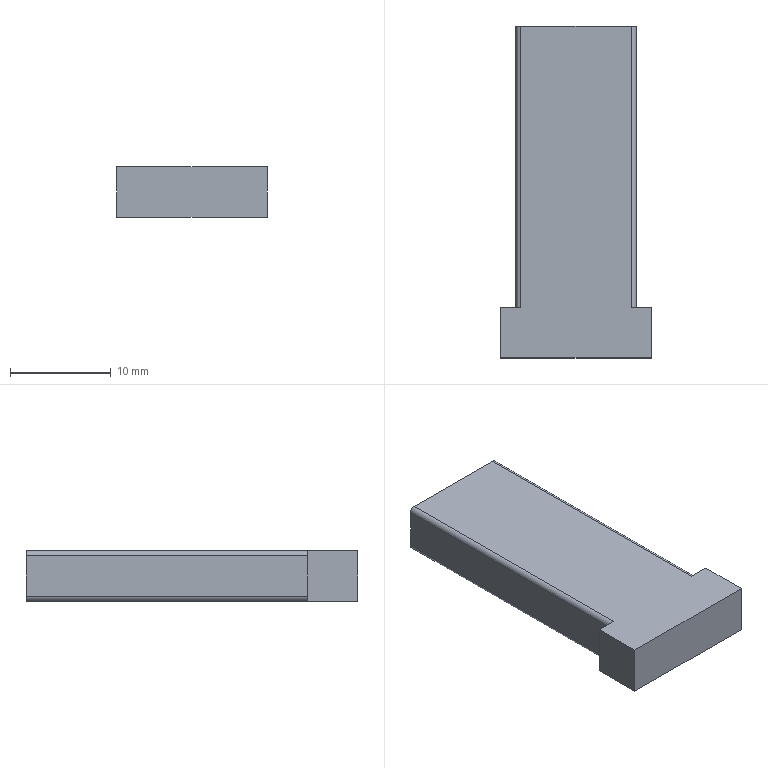Part | SolidWorks | features Extrusion 1, Fillet 1, ICE 1 | 1 solid | 14 faces | box 15 x 33 x 5 mm | volume 2049 mm3 | plane 10 | cylinder 4 | commonest cylinder face diameters 1 x4
STEP:
#1=CARTESIAN_POINT('',(-6.,-49.77,-2.));
#2=VERTEX_POINT('',#1);
#3=CARTESIAN_POINT('',(-6.,-49.77,2.));
#4=VERTEX_POINT('',#3);
#5=CARTESIAN_POINT('',(-6.,-49.77,2.5));
#6=DIRECTION('',(0.,0.,1.));
#7=VECTOR('',#6,1000.);
#8=LINE('',#5,#7);
#9=EDGE_CURVE('',#2,#4,#8,.T.);
#10=ORIENTED_EDGE('',*,*,#9,.F.);
#11=CARTESIAN_POINT('',(-5.5,-49.77,-2.5));
#12=VERTEX_POINT('',#11);
#13=CARTESIAN_POINT('',(-5.5,-49.77,-2.));
#14=DIRECTION('',(0.,-1.,0.));
#15=DIRECTION('',(0.,0.,-1.));
#16=AXIS2_PLACEMENT_3D('',#13,#14,#15);
#17=CIRCLE('',#16,0.5);
#18=EDGE_CURVE('',#2,#12,#17,.T.);
#19=ORIENTED_EDGE('',*,*,#18,.T.);
#20=CARTESIAN_POINT('',(-7.5,-49.77,-2.5));
#21=VERTEX_POINT('',#20);
#22=CARTESIAN_POINT('',(7.5,-49.77,-2.5));
#23=DIRECTION('',(-1.,0.,0.));
#24=VECTOR('',#23,1000.);
#25=LINE('',#22,#24);
#26=EDGE_CURVE('',#12,#21,#25,.T.);
#27=ORIENTED_EDGE('',*,*,#26,.T.);
#28=CARTESIAN_POINT('',(-7.5,-49.77,2.5));
#29=VERTEX_POINT('',#28);
#30=CARTESIAN_POINT('',(-7.5,-49.77,2.5));
#31=DIRECTION('',(0.,0.,-1.));
#32=VECTOR('',#31,1000.);
#33=LINE('',#30,#32);
#34=EDGE_CURVE('',#29,#21,#33,.T.);
#35=ORIENTED_EDGE('',*,*,#34,.F.);
#36=CARTESIAN_POINT('',(-5.5,-49.77,2.5));
#37=VERTEX_POINT('',#36);
#38=CARTESIAN_POINT('',(7.5,-49.77,2.5));
#39=DIRECTION('',(-1.,0.,0.));
#40=VECTOR('',#39,1000.);
#41=LINE('',#38,#40);
#42=EDGE_CURVE('',#37,#29,#41,.T.);
#43=ORIENTED_EDGE('',*,*,#42,.F.);
#44=CARTESIAN_POINT('',(-5.5,-49.77,2.));
#45=DIRECTION('',(0.,-1.,0.));
#46=DIRECTION('',(0.,0.,-1.));
#47=AXIS2_PLACEMENT_3D('',#44,#45,#46);
#48=CIRCLE('',#47,0.5);
#49=EDGE_CURVE('',#37,#4,#48,.T.);
#50=ORIENTED_EDGE('',*,*,#49,.T.);
#51=EDGE_LOOP('',(#10,#19,#27,#35,#43,#50));
#52=FACE_OUTER_BOUND('',#51,.T.);
#53=CARTESIAN_POINT('',(7.5,-49.77,2.5));
#54=DIRECTION('',(0.,-1.,0.));
#55=DIRECTION('',(0.,0.,-1.));
#56=AXIS2_PLACEMENT_3D('',#53,#54,#55);
#57=PLANE('',#56);
#58=ADVANCED_FACE('',(#52),#57,.F.);
#59=CARTESIAN_POINT('',(6.,-49.77,2.));
#60=VERTEX_POINT('',#59);
#61=CARTESIAN_POINT('',(6.,-49.77,-2.));
#62=VERTEX_POINT('',#61);
#63=CARTESIAN_POINT('',(6.,-49.77,2.5));
#64=DIRECTION('',(0.,0.,-1.));
#65=VECTOR('',#64,1000.);
#66=LINE('',#63,#65);
#67=EDGE_CURVE('',#60,#62,#66,.T.);
#68=ORIENTED_EDGE('',*,*,#67,.F.);
#69=CARTESIAN_POINT('',(5.5,-49.77,2.5));
#70=VERTEX_POINT('',#69);
#71=CARTESIAN_POINT('',(5.5,-49.77,2.));
#72=DIRECTION('',(0.,-1.,0.));
#73=DIRECTION('',(0.,0.,-1.));
#74=AXIS2_PLACEMENT_3D('',#71,#72,#73);
#75=CIRCLE('',#74,0.5);
#76=EDGE_CURVE('',#60,#70,#75,.T.);
#77=ORIENTED_EDGE('',*,*,#76,.T.);
#78=CARTESIAN_POINT('',(7.5,-49.77,2.5));
#79=VERTEX_POINT('',#78);
#80=CARTESIAN_POINT('',(7.5,-49.77,2.5));
#81=DIRECTION('',(-1.,0.,0.));
#82=VECTOR('',#81,1000.);
#83=LINE('',#80,#82);
#84=EDGE_CURVE('',#79,#70,#83,.T.);
#85=ORIENTED_EDGE('',*,*,#84,.F.);
#86=CARTESIAN_POINT('',(7.5,-49.77,-2.5));
#87=VERTEX_POINT('',#86);
#88=CARTESIAN_POINT('',(7.5,-49.77,2.5));
#89=DIRECTION('',(0.,0.,-1.));
#90=VECTOR('',#89,1000.);
#91=LINE('',#88,#90);
#92=EDGE_CURVE('',#79,#87,#91,.T.);
#93=ORIENTED_EDGE('',*,*,#92,.T.);
#94=CARTESIAN_POINT('',(5.5,-49.77,-2.5));
#95=VERTEX_POINT('',#94);
#96=CARTESIAN_POINT('',(7.5,-49.77,-2.5));
#97=DIRECTION('',(-1.,0.,0.));
#98=VECTOR('',#97,1000.);
#99=LINE('',#96,#98);
#100=EDGE_CURVE('',#87,#95,#99,.T.);
#101=ORIENTED_EDGE('',*,*,#100,.T.);
#102=CARTESIAN_POINT('',(5.5,-49.77,-2.));
#103=DIRECTION('',(0.,-1.,0.));
#104=DIRECTION('',(0.,0.,-1.));
#105=AXIS2_PLACEMENT_3D('',#102,#103,#104);
#106=CIRCLE('',#105,0.5);
#107=EDGE_CURVE('',#95,#62,#106,.T.);
#108=ORIENTED_EDGE('',*,*,#107,.T.);
#109=EDGE_LOOP('',(#68,#77,#85,#93,#101,#108));
#110=FACE_OUTER_BOUND('',#109,.T.);
#111=CARTESIAN_POINT('',(7.5,-49.77,2.5));
#112=DIRECTION('',(0.,-1.,0.));
#113=DIRECTION('',(0.,0.,-1.));
#114=AXIS2_PLACEMENT_3D('',#111,#112,#113);
#115=PLANE('',#114);
#116=ADVANCED_FACE('',(#110),#115,.F.);
#117=CARTESIAN_POINT('',(-7.5,-54.77,-2.5));
#118=VERTEX_POINT('',#117);
#119=CARTESIAN_POINT('',(-7.5,-54.77,-2.5));
#120=DIRECTION('',(0.,-1.,0.));
#121=VECTOR('',#120,1000.);
#122=LINE('',#119,#121);
#123=EDGE_CURVE('',#21,#118,#122,.T.);
#124=ORIENTED_EDGE('',*,*,#123,.T.);
#125=CARTESIAN_POINT('',(-7.5,-54.77,2.5));
#126=VERTEX_POINT('',#125);
#127=CARTESIAN_POINT('',(-7.5,-54.77,2.5));
#128=DIRECTION('',(0.,0.,-1.));
#129=VECTOR('',#128,1000.);
#130=LINE('',#127,#129);
#131=EDGE_CURVE('',#126,#118,#130,.T.);
#132=ORIENTED_EDGE('',*,*,#131,.F.);
#133=CARTESIAN_POINT('',(-7.5,-54.77,2.5));
#134=DIRECTION('',(0.,-1.,0.));
#135=VECTOR('',#134,1000.);
#136=LINE('',#133,#135);
#137=EDGE_CURVE('',#29,#126,#136,.T.);
#138=ORIENTED_EDGE('',*,*,#137,.F.);
#139=ORIENTED_EDGE('',*,*,#34,.T.);
#140=EDGE_LOOP('',(#124,#132,#138,#139));
#141=FACE_OUTER_BOUND('',#140,.T.);
#142=CARTESIAN_POINT('',(-7.5,-54.77,2.5));
#143=DIRECTION('',(1.,0.,0.));
#144=DIRECTION('',(0.,1.,0.));
#145=AXIS2_PLACEMENT_3D('',#142,#143,#144);
#146=PLANE('',#145);
#147=ADVANCED_FACE('',(#141),#146,.F.);
#148=CARTESIAN_POINT('',(7.5,-54.77,-2.5));
#149=VERTEX_POINT('',#148);
#150=CARTESIAN_POINT('',(7.5,-54.77,-2.5));
#151=DIRECTION('',(1.,0.,0.));
#152=VECTOR('',#151,1000.);
#153=LINE('',#150,#152);
#154=EDGE_CURVE('',#118,#149,#153,.T.);
#155=ORIENTED_EDGE('',*,*,#154,.T.);
#156=CARTESIAN_POINT('',(7.5,-54.77,2.5));
#157=VERTEX_POINT('',#156);
#158=CARTESIAN_POINT('',(7.5,-54.77,2.5));
#159=DIRECTION('',(0.,0.,-1.));
#160=VECTOR('',#159,1000.);
#161=LINE('',#158,#160);
#162=EDGE_CURVE('',#157,#149,#161,.T.);
#163=ORIENTED_EDGE('',*,*,#162,.F.);
#164=CARTESIAN_POINT('',(7.5,-54.77,2.5));
#165=DIRECTION('',(1.,0.,0.));
#166=VECTOR('',#165,1000.);
#167=LINE('',#164,#166);
#168=EDGE_CURVE('',#126,#157,#167,.T.);
#169=ORIENTED_EDGE('',*,*,#168,.F.);
#170=ORIENTED_EDGE('',*,*,#131,.T.);
#171=EDGE_LOOP('',(#155,#163,#169,#170));
#172=FACE_OUTER_BOUND('',#171,.T.);
#173=CARTESIAN_POINT('',(7.5,-54.77,2.5));
#174=DIRECTION('',(0.,1.,0.));
#175=DIRECTION('',(0.,0.,1.));
#176=AXIS2_PLACEMENT_3D('',#173,#174,#175);
#177=PLANE('',#176);
#178=ADVANCED_FACE('',(#172),#177,.F.);
#179=CARTESIAN_POINT('',(7.5,-54.77,-2.5));
#180=DIRECTION('',(0.,1.,0.));
#181=VECTOR('',#180,1000.);
#182=LINE('',#179,#181);
#183=EDGE_CURVE('',#149,#87,#182,.T.);
#184=ORIENTED_EDGE('',*,*,#183,.T.);
#185=ORIENTED_EDGE('',*,*,#92,.F.);
#186=CARTESIAN_POINT('',(7.5,-54.77,2.5));
#187=DIRECTION('',(0.,1.,0.));
#188=VECTOR('',#187,1000.);
#189=LINE('',#186,#188);
#190=EDGE_CURVE('',#157,#79,#189,.T.);
#191=ORIENTED_EDGE('',*,*,#190,.F.);
#192=ORIENTED_EDGE('',*,*,#162,.T.);
#193=EDGE_LOOP('',(#184,#185,#191,#192));
#194=FACE_OUTER_BOUND('',#193,.T.);
#195=CARTESIAN_POINT('',(7.5,-54.77,2.5));
#196=DIRECTION('',(-1.,0.,0.));
#197=DIRECTION('',(0.,0.,1.));
#198=AXIS2_PLACEMENT_3D('',#195,#196,#197);
#199=PLANE('',#198);
#200=ADVANCED_FACE('',(#194),#199,.F.);
#201=CARTESIAN_POINT('',(-5.5,-21.77,2.5));
#202=VERTEX_POINT('',#201);
#203=CARTESIAN_POINT('',(5.5,-21.77,2.5));
#204=VERTEX_POINT('',#203);
#205=CARTESIAN_POINT('',(6.,-21.77,2.5));
#206=DIRECTION('',(1.,0.,0.));
#207=VECTOR('',#206,1000.);
#208=LINE('',#205,#207);
#209=EDGE_CURVE('',#202,#204,#208,.T.);
#210=ORIENTED_EDGE('',*,*,#209,.F.);
#211=CARTESIAN_POINT('',(-5.5,-49.77,2.5));
#212=DIRECTION('',(0.,-1.,0.));
#213=VECTOR('',#212,1000.);
#214=LINE('',#211,#213);
#215=EDGE_CURVE('',#202,#37,#214,.T.);
#216=ORIENTED_EDGE('',*,*,#215,.T.);
#217=ORIENTED_EDGE('',*,*,#42,.T.);
#218=ORIENTED_EDGE('',*,*,#137,.T.);
#219=ORIENTED_EDGE('',*,*,#168,.T.);
#220=ORIENTED_EDGE('',*,*,#190,.T.);
#221=ORIENTED_EDGE('',*,*,#84,.T.);
#222=CARTESIAN_POINT('',(5.5,-21.77,2.5));
#223=DIRECTION('',(0.,1.,0.));
#224=VECTOR('',#223,1000.);
#225=LINE('',#222,#224);
#226=EDGE_CURVE('',#70,#204,#225,.T.);
#227=ORIENTED_EDGE('',*,*,#226,.T.);
#228=EDGE_LOOP('',(#210,#216,#217,#218,#219,#220,#221,#227));
#229=FACE_OUTER_BOUND('',#228,.T.);
#230=CARTESIAN_POINT('',(0.,0.,2.5));
#231=DIRECTION('',(0.,0.,1.));
#232=DIRECTION('',(1.,0.,0.));
#233=AXIS2_PLACEMENT_3D('',#230,#231,#232);
#234=PLANE('',#233);
#235=ADVANCED_FACE('',(#229),#234,.T.);
#236=ORIENTED_EDGE('',*,*,#26,.F.);
#237=CARTESIAN_POINT('',(-5.5,-21.77,-2.5));
#238=VERTEX_POINT('',#237);
#239=CARTESIAN_POINT('',(-5.5,0.,-2.5));
#240=DIRECTION('',(0.,1.,0.));
#241=VECTOR('',#240,1000.);
#242=LINE('',#239,#241);
#243=EDGE_CURVE('',#12,#238,#242,.T.);
#244=ORIENTED_EDGE('',*,*,#243,.T.);
#245=CARTESIAN_POINT('',(5.5,-21.77,-2.5));
#246=VERTEX_POINT('',#245);
#247=CARTESIAN_POINT('',(6.,-21.77,-2.5));
#248=DIRECTION('',(-1.,0.,0.));
#249=VECTOR('',#248,1000.);
#250=LINE('',#247,#249);
#251=EDGE_CURVE('',#246,#238,#250,.T.);
#252=ORIENTED_EDGE('',*,*,#251,.F.);
#253=CARTESIAN_POINT('',(5.5,0.,-2.5));
#254=DIRECTION('',(0.,-1.,0.));
#255=VECTOR('',#254,1000.);
#256=LINE('',#253,#255);
#257=EDGE_CURVE('',#246,#95,#256,.T.);
#258=ORIENTED_EDGE('',*,*,#257,.T.);
#259=ORIENTED_EDGE('',*,*,#100,.F.);
#260=ORIENTED_EDGE('',*,*,#183,.F.);
#261=ORIENTED_EDGE('',*,*,#154,.F.);
#262=ORIENTED_EDGE('',*,*,#123,.F.);
#263=EDGE_LOOP('',(#236,#244,#252,#258,#259,#260,#261,#262));
#264=FACE_OUTER_BOUND('',#263,.T.);
#265=CARTESIAN_POINT('',(0.,0.,-2.5));
#266=DIRECTION('',(0.,0.,1.));
#267=DIRECTION('',(1.,0.,0.));
#268=AXIS2_PLACEMENT_3D('',#265,#266,#267);
#269=PLANE('',#268);
#270=ADVANCED_FACE('',(#264),#269,.F.);
#271=ORIENTED_EDGE('',*,*,#9,.T.);
#272=CARTESIAN_POINT('',(-6.,-21.77,2.));
#273=VERTEX_POINT('',#272);
#274=CARTESIAN_POINT('',(-6.,-21.77,2.));
#275=DIRECTION('',(0.,1.,0.));
#276=VECTOR('',#275,1000.);
#277=LINE('',#274,#276);
#278=EDGE_CURVE('',#4,#273,#277,.T.);
#279=ORIENTED_EDGE('',*,*,#278,.T.);
#280=CARTESIAN_POINT('',(-6.,-21.77,-2.));
#281=VERTEX_POINT('',#280);
#282=CARTESIAN_POINT('',(-6.,-21.77,2.5));
#283=DIRECTION('',(0.,0.,1.));
#284=VECTOR('',#283,1000.);
#285=LINE('',#282,#284);
#286=EDGE_CURVE('',#281,#273,#285,.T.);
#287=ORIENTED_EDGE('',*,*,#286,.F.);
#288=CARTESIAN_POINT('',(-6.,-21.77,-2.));
#289=DIRECTION('',(0.,-1.,0.));
#290=VECTOR('',#289,1000.);
#291=LINE('',#288,#290);
#292=EDGE_CURVE('',#281,#2,#291,.T.);
#293=ORIENTED_EDGE('',*,*,#292,.T.);
#294=EDGE_LOOP('',(#271,#279,#287,#293));
#295=FACE_OUTER_BOUND('',#294,.T.);
#296=CARTESIAN_POINT('',(-6.,-21.77,2.5));
#297=DIRECTION('',(1.,0.,0.));
#298=DIRECTION('',(0.,0.,-1.));
#299=AXIS2_PLACEMENT_3D('',#296,#297,#298);
#300=PLANE('',#299);
#301=ADVANCED_FACE('',(#295),#300,.F.);
#302=ORIENTED_EDGE('',*,*,#67,.T.);
#303=CARTESIAN_POINT('',(6.,-21.77,-2.));
#304=VERTEX_POINT('',#303);
#305=CARTESIAN_POINT('',(6.,-21.77,-2.));
#306=DIRECTION('',(0.,1.,0.));
#307=VECTOR('',#306,1000.);
#308=LINE('',#305,#307);
#309=EDGE_CURVE('',#62,#304,#308,.T.);
#310=ORIENTED_EDGE('',*,*,#309,.T.);
#311=CARTESIAN_POINT('',(6.,-21.77,2.));
#312=VERTEX_POINT('',#311);
#313=CARTESIAN_POINT('',(6.,-21.77,2.5));
#314=DIRECTION('',(0.,0.,-1.));
#315=VECTOR('',#314,1000.);
#316=LINE('',#313,#315);
#317=EDGE_CURVE('',#312,#304,#316,.T.);
#318=ORIENTED_EDGE('',*,*,#317,.F.);
#319=CARTESIAN_POINT('',(6.,-49.77,2.));
#320=DIRECTION('',(0.,-1.,0.));
#321=VECTOR('',#320,1000.);
#322=LINE('',#319,#321);
#323=EDGE_CURVE('',#312,#60,#322,.T.);
#324=ORIENTED_EDGE('',*,*,#323,.T.);
#325=EDGE_LOOP('',(#302,#310,#318,#324));
#326=FACE_OUTER_BOUND('',#325,.T.);
#327=CARTESIAN_POINT('',(6.,-21.77,2.5));
#328=DIRECTION('',(-1.,0.,0.));
#329=DIRECTION('',(0.,0.,1.));
#330=AXIS2_PLACEMENT_3D('',#327,#328,#329);
#331=PLANE('',#330);
#332=ADVANCED_FACE('',(#326),#331,.F.);
#333=ORIENTED_EDGE('',*,*,#286,.T.);
#334=CARTESIAN_POINT('',(-5.5,-21.77,2.));
#335=DIRECTION('',(0.,1.,0.));
#336=DIRECTION('',(0.,0.,1.));
#337=AXIS2_PLACEMENT_3D('',#334,#335,#336);
#338=CIRCLE('',#337,0.5);
#339=EDGE_CURVE('',#273,#202,#338,.T.);
#340=ORIENTED_EDGE('',*,*,#339,.T.);
#341=ORIENTED_EDGE('',*,*,#209,.T.);
#342=CARTESIAN_POINT('',(5.5,-21.77,2.));
#343=DIRECTION('',(0.,1.,0.));
#344=DIRECTION('',(0.,0.,1.));
#345=AXIS2_PLACEMENT_3D('',#342,#343,#344);
#346=CIRCLE('',#345,0.5);
#347=EDGE_CURVE('',#204,#312,#346,.T.);
#348=ORIENTED_EDGE('',*,*,#347,.T.);
#349=ORIENTED_EDGE('',*,*,#317,.T.);
#350=CARTESIAN_POINT('',(5.5,-21.77,-2.));
#351=DIRECTION('',(0.,1.,0.));
#352=DIRECTION('',(0.,0.,1.));
#353=AXIS2_PLACEMENT_3D('',#350,#351,#352);
#354=CIRCLE('',#353,0.5);
#355=EDGE_CURVE('',#304,#246,#354,.T.);
#356=ORIENTED_EDGE('',*,*,#355,.T.);
#357=ORIENTED_EDGE('',*,*,#251,.T.);
#358=CARTESIAN_POINT('',(-5.5,-21.77,-2.));
#359=DIRECTION('',(0.,1.,0.));
#360=DIRECTION('',(0.,0.,1.));
#361=AXIS2_PLACEMENT_3D('',#358,#359,#360);
#362=CIRCLE('',#361,0.5);
#363=EDGE_CURVE('',#238,#281,#362,.T.);
#364=ORIENTED_EDGE('',*,*,#363,.T.);
#365=EDGE_LOOP('',(#333,#340,#341,#348,#349,#356,#357,#364));
#366=FACE_OUTER_BOUND('',#365,.T.);
#367=CARTESIAN_POINT('',(0.,-21.77,0.));
#368=DIRECTION('',(0.,1.,0.));
#369=DIRECTION('',(0.,0.,1.));
#370=AXIS2_PLACEMENT_3D('',#367,#368,#369);
#371=PLANE('',#370);
#372=ADVANCED_FACE('',(#366),#371,.T.);
#373=ORIENTED_EDGE('',*,*,#339,.F.);
#374=ORIENTED_EDGE('',*,*,#278,.F.);
#375=ORIENTED_EDGE('',*,*,#49,.F.);
#376=ORIENTED_EDGE('',*,*,#215,.F.);
#377=EDGE_LOOP('',(#373,#374,#375,#376));
#378=FACE_OUTER_BOUND('',#377,.T.);
#379=CARTESIAN_POINT('',(-5.5,0.,2.));
#380=DIRECTION('',(0.,1.,0.));
#381=DIRECTION('',(0.,0.,1.));
#382=AXIS2_PLACEMENT_3D('',#379,#380,#381);
#383=CYLINDRICAL_SURFACE('',#382,0.5);
#384=ADVANCED_FACE('',(#378),#383,.T.);
#385=ORIENTED_EDGE('',*,*,#363,.F.);
#386=ORIENTED_EDGE('',*,*,#243,.F.);
#387=ORIENTED_EDGE('',*,*,#18,.F.);
#388=ORIENTED_EDGE('',*,*,#292,.F.);
#389=EDGE_LOOP('',(#385,#386,#387,#388));
#390=FACE_OUTER_BOUND('',#389,.T.);
#391=CARTESIAN_POINT('',(-5.5,-21.77,-2.));
#392=DIRECTION('',(0.,-1.,0.));
#393=DIRECTION('',(0.,0.,-1.));
#394=AXIS2_PLACEMENT_3D('',#391,#392,#393);
#395=CYLINDRICAL_SURFACE('',#394,0.5);
#396=ADVANCED_FACE('',(#390),#395,.T.);
#397=ORIENTED_EDGE('',*,*,#355,.F.);
#398=ORIENTED_EDGE('',*,*,#309,.F.);
#399=ORIENTED_EDGE('',*,*,#107,.F.);
#400=ORIENTED_EDGE('',*,*,#257,.F.);
#401=EDGE_LOOP('',(#397,#398,#399,#400));
#402=FACE_OUTER_BOUND('',#401,.T.);
#403=CARTESIAN_POINT('',(5.5,0.,-2.));
#404=DIRECTION('',(0.,-1.,0.));
#405=DIRECTION('',(0.,0.,-1.));
#406=AXIS2_PLACEMENT_3D('',#403,#404,#405);
#407=CYLINDRICAL_SURFACE('',#406,0.5);
#408=ADVANCED_FACE('',(#402),#407,.T.);
#409=ORIENTED_EDGE('',*,*,#347,.F.);
#410=ORIENTED_EDGE('',*,*,#226,.F.);
#411=ORIENTED_EDGE('',*,*,#76,.F.);
#412=ORIENTED_EDGE('',*,*,#323,.F.);
#413=EDGE_LOOP('',(#409,#410,#411,#412));
#414=FACE_OUTER_BOUND('',#413,.T.);
#415=CARTESIAN_POINT('',(5.5,-21.77,2.));
#416=DIRECTION('',(0.,1.,0.));
#417=DIRECTION('',(0.,0.,1.));
#418=AXIS2_PLACEMENT_3D('',#415,#416,#417);
#419=CYLINDRICAL_SURFACE('',#418,0.5);
#420=ADVANCED_FACE('',(#414),#419,.T.);
#421=CLOSED_SHELL('',(#58,#116,#147,#178,#200,#235,#270,#301,#332,#372,#384,#396,#408,#420));
#422=MANIFOLD_SOLID_BREP('',#421);
#423=CARTESIAN_POINT('',(0.,0.,0.));
#424=DIRECTION('',(0.,0.,1.));
#425=DIRECTION('',(1.,0.,0.));
#426=AXIS2_PLACEMENT_3D('',#423,#424,#425);
#427=(LENGTH_UNIT()NAMED_UNIT(*)SI_UNIT(.MILLI.,.METRE.));
#428=UNCERTAINTY_MEASURE_WITH_UNIT(LENGTH_MEASURE(0.00001),#427,'','');
#429=(NAMED_UNIT(*)PLANE_ANGLE_UNIT()SI_UNIT($,.RADIAN.));
#430=(NAMED_UNIT(*)SI_UNIT($,.STERADIAN.)SOLID_ANGLE_UNIT());
#431=(GEOMETRIC_REPRESENTATION_CONTEXT(3)GLOBAL_UNCERTAINTY_ASSIGNED_CONTEXT((#428))GLOBAL_UNIT_ASSIGNED_CONTEXT((#427,#429,#430))REPRESENTATION_CONTEXT('',''));
#432=ADVANCED_BREP_SHAPE_REPRESENTATION('',(#422,#426),#431);